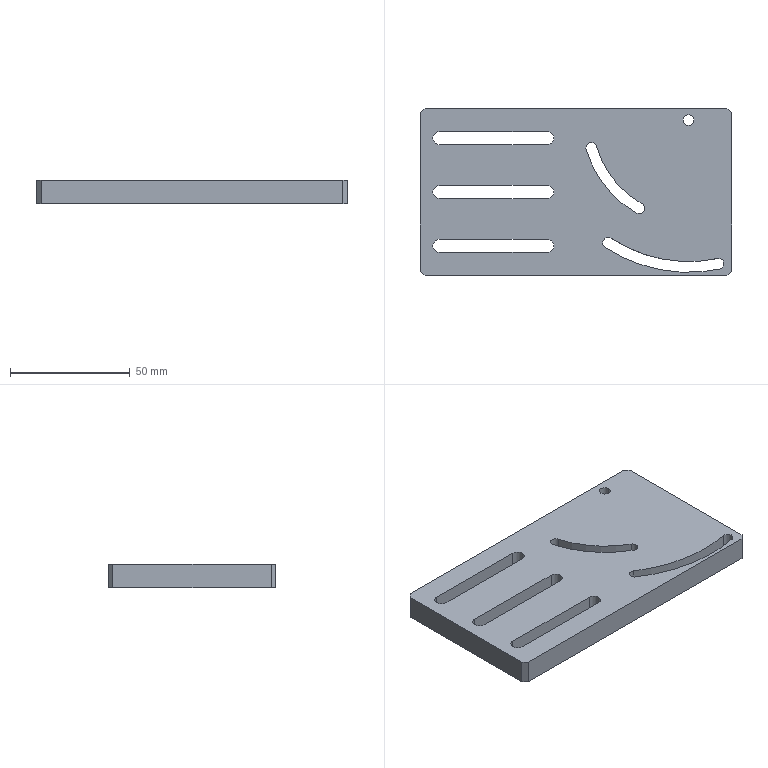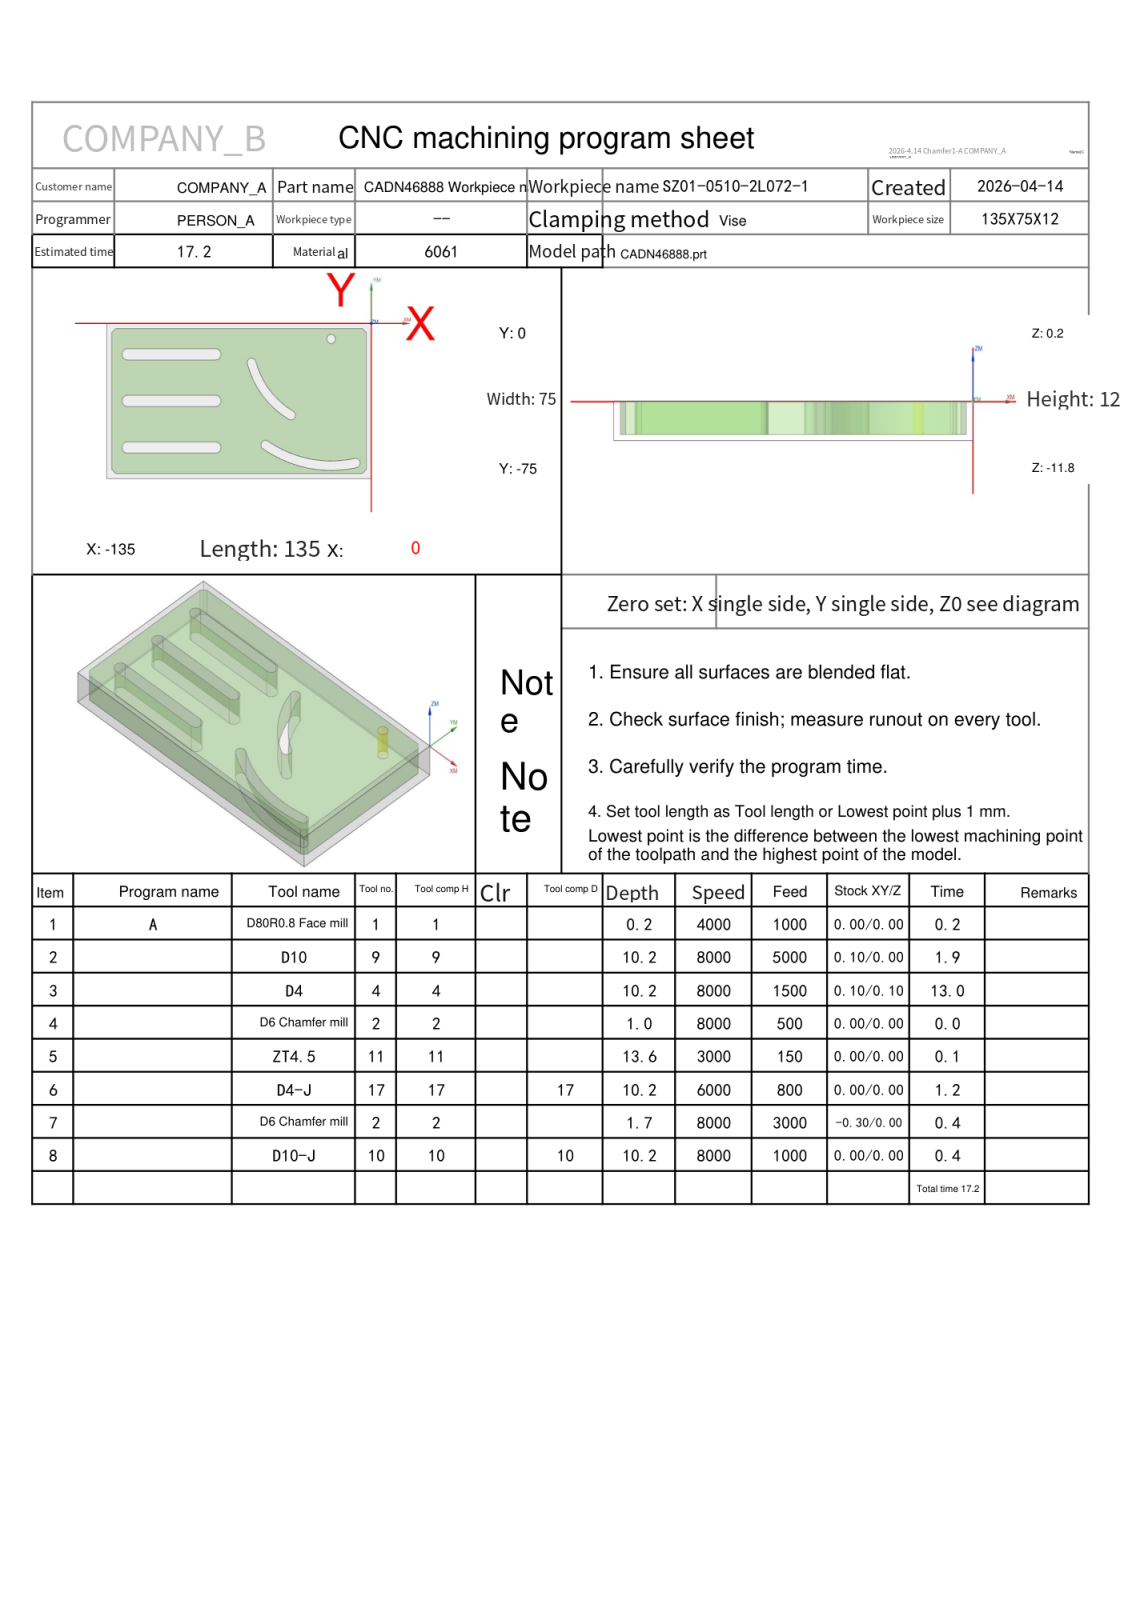NC program | NX | posted by the shop | part box 130 x 70 x 10 mm
Lines 1 to 447 of 2533:
%
O0001
(Machine time: 14.74 MIN)
(===Total Tool:7===)
(T1=D80R0.8 Face mill D=80.  R=0.8  D-  H01 Z=0.    )
(T9=D10     D=10.  R=0.   D-  H09 Z=-10.  )
(T2=D6 Chamfer mill   D=6.   R=0.   D-  H02 Z=-1.5  )
(T11=ZT4.5  D=4.5  DR_a=118 D-  H11 Z=-13.35)
(T4=D4      D=4.   R=0.   D-  H04 Z=-10.  )
(T17=D4-J   D=4.   R=0.   D17 H17 Z=-10.  )
(T10=D10-J  D=10.  R=0.   D10 H10 Z=-10.  )
G80 G90 G17 G49 G40
G91 G28 Z0
M01
N1 T01 M06
(D80R0.8 Face mill  D=80. R=0.8 H=01 ce=0.00 di=0.00)
G00 G90 G54 X-177.5 Y-37.5 M03 S4000
G43 H01 Z20.
M08
Z2.
G01 Z0.0 F1000.
X-172.5
X37.5
X42.5
Z2.
G00 Z20.
G91 G28 Z0.0
M05
M09
G91 G28 Z0.0
M01
N2 T09 M06
(D10  D=10. R=0. H=09 ce=0.10 di=0.00)
G00 G90 G54 X-67.5 Y2.6 M03 S8000
G43 H09 Z20.
M08
Z.5
G01 X-4.5 Z.426 F5000.
G02 X-.894 Y1.106 Z.422 I0.0 J-5.1
G01 X1.106 Y-.894 Z.418
G02 X2.6 Y-4.5 Z.414 I-3.606 J-3.606
G01 Y-70.5 Z.336
G02 X1.106 Y-74.106 Z.332 I-5.1 J0.0
G01 X-.894 Y-76.106 Z.328
G02 X-4.5 Y-77.6 Z.324 I-3.606 J3.606
G01 X-130.5 Z.176
G02 X-134.106 Y-76.106 Z.172 I0.0 J5.1
G01 X-136.106 Y-74.106 Z.168
G02 X-137.6 Y-70.5 Z.164 I3.606 J3.606
G01 Y-4.5 Z.086
G02 X-136.106 Y-.894 Z.082 I5.1 J0.0
G01 X-134.106 Y1.106 Z.078
G02 X-130.5 Y2.6 Z.074 I3.606 J-3.606
G01 X-4.5 Z-.074
G02 X-.894 Y1.106 Z-.078 I0.0 J-5.1
G01 X1.106 Y-.894 Z-.082
G02 X2.6 Y-4.5 Z-.086 I-3.606 J-3.606
G01 Y-70.5 Z-.164
G02 X1.106 Y-74.106 Z-.168 I-5.1 J0.0
G01 X-.894 Y-76.106 Z-.172
G02 X-4.5 Y-77.6 Z-.176 I-3.606 J3.606
G01 X-130.5 Z-.324
G02 X-134.106 Y-76.106 Z-.328 I0.0 J5.1
G01 X-136.106 Y-74.106 Z-.332
G02 X-137.6 Y-70.5 Z-.336 I3.606 J3.606
G01 Y-4.5 Z-.414
G02 X-136.106 Y-.894 Z-.418 I5.1 J0.0
G01 X-134.106 Y1.106 Z-.422
G02 X-130.5 Y2.6 Z-.426 I3.606 J-3.606
G01 X-4.5 Z-.574
G02 X-.894 Y1.106 Z-.578 I0.0 J-5.1
G01 X1.106 Y-.894 Z-.582
G02 X2.6 Y-4.5 Z-.586 I-3.606 J-3.606
G01 Y-70.5 Z-.664
G02 X1.106 Y-74.106 Z-.668 I-5.1 J0.0
G01 X-.894 Y-76.106 Z-.672
G02 X-4.5 Y-77.6 Z-.676 I-3.606 J3.606
G01 X-130.5 Z-.824
G02 X-134.106 Y-76.106 Z-.828 I0.0 J5.1
G01 X-136.106 Y-74.106 Z-.832
G02 X-137.6 Y-70.5 Z-.836 I3.606 J3.606
G01 Y-4.5 Z-.914
G02 X-136.106 Y-.894 Z-.918 I5.1 J0.0
G01 X-134.106 Y1.106 Z-.922
G02 X-130.5 Y2.6 Z-.926 I3.606 J-3.606
G01 X-4.5 Z-1.074
G02 X-.894 Y1.106 Z-1.078 I0.0 J-5.1
G01 X1.106 Y-.894 Z-1.082
G02 X2.6 Y-4.5 Z-1.086 I-3.606 J-3.606
G01 Y-70.5 Z-1.164
G02 X1.106 Y-74.106 Z-1.168 I-5.1 J0.0
G01 X-.894 Y-76.106 Z-1.172
G02 X-4.5 Y-77.6 Z-1.176 I-3.606 J3.606
G01 X-130.5 Z-1.324
G02 X-134.106 Y-76.106 Z-1.328 I0.0 J5.1
G01 X-136.106 Y-74.106 Z-1.332
G02 X-137.6 Y-70.5 Z-1.336 I3.606 J3.606
G01 Y-4.5 Z-1.414
G02 X-136.106 Y-.894 Z-1.418 I5.1 J0.0
G01 X-134.106 Y1.106 Z-1.422
G02 X-130.5 Y2.6 Z-1.426 I3.606 J-3.606
G01 X-4.5 Z-1.574
G02 X-.894 Y1.106 Z-1.578 I0.0 J-5.1
G01 X1.106 Y-.894 Z-1.582
G02 X2.6 Y-4.5 Z-1.586 I-3.606 J-3.606
G01 Y-70.5 Z-1.664
G02 X1.106 Y-74.106 Z-1.668 I-5.1 J0.0
G01 X-.894 Y-76.106 Z-1.672
G02 X-4.5 Y-77.6 Z-1.676 I-3.606 J3.606
G01 X-130.5 Z-1.824
G02 X-134.106 Y-76.106 Z-1.828 I0.0 J5.1
G01 X-136.106 Y-74.106 Z-1.832
G02 X-137.6 Y-70.5 Z-1.836 I3.606 J3.606
G01 Y-4.5 Z-1.914
G02 X-136.106 Y-.894 Z-1.918 I5.1 J0.0
G01 X-134.106 Y1.106 Z-1.922
G02 X-130.5 Y2.6 Z-1.926 I3.606 J-3.606
G01 X-4.5 Z-2.074
G02 X-.894 Y1.106 Z-2.078 I0.0 J-5.1
G01 X1.106 Y-.894 Z-2.082
G02 X2.6 Y-4.5 Z-2.086 I-3.606 J-3.606
G01 Y-70.5 Z-2.164
G02 X1.106 Y-74.106 Z-2.168 I-5.1 J0.0
G01 X-.894 Y-76.106 Z-2.172
G02 X-4.5 Y-77.6 Z-2.176 I-3.606 J3.606
G01 X-130.5 Z-2.324
G02 X-134.106 Y-76.106 Z-2.328 I0.0 J5.1
G01 X-136.106 Y-74.106 Z-2.332
G02 X-137.6 Y-70.5 Z-2.336 I3.606 J3.606
G01 Y-4.5 Z-2.414
G02 X-136.106 Y-.894 Z-2.418 I5.1 J0.0
G01 X-134.106 Y1.106 Z-2.422
G02 X-130.5 Y2.6 Z-2.426 I3.606 J-3.606
G01 X-4.5 Z-2.574
G02 X-.894 Y1.106 Z-2.578 I0.0 J-5.1
G01 X1.106 Y-.894 Z-2.582
G02 X2.6 Y-4.5 Z-2.586 I-3.606 J-3.606
G01 Y-70.5 Z-2.664
G02 X1.106 Y-74.106 Z-2.668 I-5.1 J0.0
G01 X-.894 Y-76.106 Z-2.672
G02 X-4.5 Y-77.6 Z-2.676 I-3.606 J3.606
G01 X-130.5 Z-2.824
G02 X-134.106 Y-76.106 Z-2.828 I0.0 J5.1
G01 X-136.106 Y-74.106 Z-2.832
G02 X-137.6 Y-70.5 Z-2.836 I3.606 J3.606
G01 Y-4.5 Z-2.914
G02 X-136.106 Y-.894 Z-2.918 I5.1 J0.0
G01 X-134.106 Y1.106 Z-2.922
G02 X-130.5 Y2.6 Z-2.926 I3.606 J-3.606
G01 X-4.5 Z-3.074
G02 X-.894 Y1.106 Z-3.078 I0.0 J-5.1
G01 X1.106 Y-.894 Z-3.082
G02 X2.6 Y-4.5 Z-3.086 I-3.606 J-3.606
G01 Y-70.5 Z-3.164
G02 X1.106 Y-74.106 Z-3.168 I-5.1 J0.0
G01 X-.894 Y-76.106 Z-3.172
G02 X-4.5 Y-77.6 Z-3.176 I-3.606 J3.606
G01 X-130.5 Z-3.324
G02 X-134.106 Y-76.106 Z-3.328 I0.0 J5.1
G01 X-136.106 Y-74.106 Z-3.332
G02 X-137.6 Y-70.5 Z-3.336 I3.606 J3.606
G01 Y-4.5 Z-3.414
G02 X-136.106 Y-.894 Z-3.418 I5.1 J0.0
G01 X-134.106 Y1.106 Z-3.422
G02 X-130.5 Y2.6 Z-3.426 I3.606 J-3.606
G01 X-4.5 Z-3.574
G02 X-.894 Y1.106 Z-3.578 I0.0 J-5.1
G01 X1.106 Y-.894 Z-3.582
G02 X2.6 Y-4.5 Z-3.586 I-3.606 J-3.606
G01 Y-70.5 Z-3.664
G02 X1.106 Y-74.106 Z-3.668 I-5.1 J0.0
G01 X-.894 Y-76.106 Z-3.672
G02 X-4.5 Y-77.6 Z-3.676 I-3.606 J3.606
G01 X-130.5 Z-3.824
G02 X-134.106 Y-76.106 Z-3.828 I0.0 J5.1
G01 X-136.106 Y-74.106 Z-3.832
G02 X-137.6 Y-70.5 Z-3.836 I3.606 J3.606
G01 Y-4.5 Z-3.914
G02 X-136.106 Y-.894 Z-3.918 I5.1 J0.0
G01 X-134.106 Y1.106 Z-3.922
G02 X-130.5 Y2.6 Z-3.926 I3.606 J-3.606
G01 X-4.5 Z-4.074
G02 X-.894 Y1.106 Z-4.078 I0.0 J-5.1
G01 X1.106 Y-.894 Z-4.082
G02 X2.6 Y-4.5 Z-4.086 I-3.606 J-3.606
G01 Y-70.5 Z-4.164
G02 X1.106 Y-74.106 Z-4.168 I-5.1 J0.0
G01 X-.894 Y-76.106 Z-4.172
G02 X-4.5 Y-77.6 Z-4.176 I-3.606 J3.606
G01 X-130.5 Z-4.324
G02 X-134.106 Y-76.106 Z-4.328 I0.0 J5.1
G01 X-136.106 Y-74.106 Z-4.332
G02 X-137.6 Y-70.5 Z-4.336 I3.606 J3.606
G01 Y-4.5 Z-4.414
G02 X-136.106 Y-.894 Z-4.418 I5.1 J0.0
G01 X-134.106 Y1.106 Z-4.422
G02 X-130.5 Y2.6 Z-4.426 I3.606 J-3.606
G01 X-4.5 Z-4.574
G02 X-.894 Y1.106 Z-4.578 I0.0 J-5.1
G01 X1.106 Y-.894 Z-4.582
G02 X2.6 Y-4.5 Z-4.586 I-3.606 J-3.606
G01 Y-70.5 Z-4.664
G02 X1.106 Y-74.106 Z-4.668 I-5.1 J0.0
G01 X-.894 Y-76.106 Z-4.672
G02 X-4.5 Y-77.6 Z-4.676 I-3.606 J3.606
G01 X-130.5 Z-4.824
G02 X-134.106 Y-76.106 Z-4.828 I0.0 J5.1
G01 X-136.106 Y-74.106 Z-4.832
G02 X-137.6 Y-70.5 Z-4.836 I3.606 J3.606
G01 Y-4.5 Z-4.914
G02 X-136.106 Y-.894 Z-4.918 I5.1 J0.0
G01 X-134.106 Y1.106 Z-4.922
G02 X-130.5 Y2.6 Z-4.926 I3.606 J-3.606
G01 X-4.5 Z-5.074
G02 X-.894 Y1.106 Z-5.078 I0.0 J-5.1
G01 X1.106 Y-.894 Z-5.082
G02 X2.6 Y-4.5 Z-5.086 I-3.606 J-3.606
G01 Y-70.5 Z-5.164
G02 X1.106 Y-74.106 Z-5.168 I-5.1 J0.0
G01 X-.894 Y-76.106 Z-5.172
G02 X-4.5 Y-77.6 Z-5.176 I-3.606 J3.606
G01 X-130.5 Z-5.324
G02 X-134.106 Y-76.106 Z-5.328 I0.0 J5.1
G01 X-136.106 Y-74.106 Z-5.332
G02 X-137.6 Y-70.5 Z-5.336 I3.606 J3.606
G01 Y-4.5 Z-5.414
G02 X-136.106 Y-.894 Z-5.418 I5.1 J0.0
G01 X-134.106 Y1.106 Z-5.422
G02 X-130.5 Y2.6 Z-5.426 I3.606 J-3.606
G01 X-4.5 Z-5.574
G02 X-.894 Y1.106 Z-5.578 I0.0 J-5.1
G01 X1.106 Y-.894 Z-5.582
G02 X2.6 Y-4.5 Z-5.586 I-3.606 J-3.606
G01 Y-70.5 Z-5.664
G02 X1.106 Y-74.106 Z-5.668 I-5.1 J0.0
G01 X-.894 Y-76.106 Z-5.672
G02 X-4.5 Y-77.6 Z-5.676 I-3.606 J3.606
G01 X-130.5 Z-5.824
G02 X-134.106 Y-76.106 Z-5.828 I0.0 J5.1
G01 X-136.106 Y-74.106 Z-5.832
G02 X-137.6 Y-70.5 Z-5.836 I3.606 J3.606
G01 Y-4.5 Z-5.914
G02 X-136.106 Y-.894 Z-5.918 I5.1 J0.0
G01 X-134.106 Y1.106 Z-5.922
G02 X-130.5 Y2.6 Z-5.926 I3.606 J-3.606
G01 X-4.5 Z-6.074
G02 X-.894 Y1.106 Z-6.078 I0.0 J-5.1
G01 X1.106 Y-.894 Z-6.082
G02 X2.6 Y-4.5 Z-6.086 I-3.606 J-3.606
G01 Y-70.5 Z-6.164
G02 X1.106 Y-74.106 Z-6.168 I-5.1 J0.0
G01 X-.894 Y-76.106 Z-6.172
G02 X-4.5 Y-77.6 Z-6.176 I-3.606 J3.606
G01 X-130.5 Z-6.324
G02 X-134.106 Y-76.106 Z-6.328 I0.0 J5.1
G01 X-136.106 Y-74.106 Z-6.332
G02 X-137.6 Y-70.5 Z-6.336 I3.606 J3.606
G01 Y-4.5 Z-6.414
G02 X-136.106 Y-.894 Z-6.418 I5.1 J0.0
G01 X-134.106 Y1.106 Z-6.422
G02 X-130.5 Y2.6 Z-6.426 I3.606 J-3.606
G01 X-4.5 Z-6.574
G02 X-.894 Y1.106 Z-6.578 I0.0 J-5.1
G01 X1.106 Y-.894 Z-6.582
G02 X2.6 Y-4.5 Z-6.586 I-3.606 J-3.606
G01 Y-70.5 Z-6.664
G02 X1.106 Y-74.106 Z-6.668 I-5.1 J0.0
G01 X-.894 Y-76.106 Z-6.672
G02 X-4.5 Y-77.6 Z-6.676 I-3.606 J3.606
G01 X-130.5 Z-6.824
G02 X-134.106 Y-76.106 Z-6.828 I0.0 J5.1
G01 X-136.106 Y-74.106 Z-6.832
G02 X-137.6 Y-70.5 Z-6.836 I3.606 J3.606
G01 Y-4.5 Z-6.914
G02 X-136.106 Y-.894 Z-6.918 I5.1 J0.0
G01 X-134.106 Y1.106 Z-6.922
G02 X-130.5 Y2.6 Z-6.926 I3.606 J-3.606
G01 X-4.5 Z-7.074
G02 X-.894 Y1.106 Z-7.078 I0.0 J-5.1
G01 X1.106 Y-.894 Z-7.082
G02 X2.6 Y-4.5 Z-7.086 I-3.606 J-3.606
G01 Y-70.5 Z-7.164
G02 X1.106 Y-74.106 Z-7.168 I-5.1 J0.0
G01 X-.894 Y-76.106 Z-7.172
G02 X-4.5 Y-77.6 Z-7.176 I-3.606 J3.606
G01 X-130.5 Z-7.324
G02 X-134.106 Y-76.106 Z-7.328 I0.0 J5.1
G01 X-136.106 Y-74.106 Z-7.332
G02 X-137.6 Y-70.5 Z-7.336 I3.606 J3.606
G01 Y-4.5 Z-7.414
G02 X-136.106 Y-.894 Z-7.418 I5.1 J0.0
G01 X-134.106 Y1.106 Z-7.422
G02 X-130.5 Y2.6 Z-7.426 I3.606 J-3.606
G01 X-4.5 Z-7.574
G02 X-.894 Y1.106 Z-7.578 I0.0 J-5.1
G01 X1.106 Y-.894 Z-7.582
G02 X2.6 Y-4.5 Z-7.586 I-3.606 J-3.606
G01 Y-70.5 Z-7.664
G02 X1.106 Y-74.106 Z-7.668 I-5.1 J0.0
G01 X-.894 Y-76.106 Z-7.672
G02 X-4.5 Y-77.6 Z-7.676 I-3.606 J3.606
G01 X-130.5 Z-7.824
G02 X-134.106 Y-76.106 Z-7.828 I0.0 J5.1
G01 X-136.106 Y-74.106 Z-7.832
G02 X-137.6 Y-70.5 Z-7.836 I3.606 J3.606
G01 Y-4.5 Z-7.914
G02 X-136.106 Y-.894 Z-7.918 I5.1 J0.0
G01 X-134.106 Y1.106 Z-7.922
G02 X-130.5 Y2.6 Z-7.926 I3.606 J-3.606
G01 X-4.5 Z-8.074
G02 X-.894 Y1.106 Z-8.078 I0.0 J-5.1
G01 X1.106 Y-.894 Z-8.082
G02 X2.6 Y-4.5 Z-8.086 I-3.606 J-3.606
G01 Y-70.5 Z-8.164
G02 X1.106 Y-74.106 Z-8.168 I-5.1 J0.0
G01 X-.894 Y-76.106 Z-8.172
G02 X-4.5 Y-77.6 Z-8.176 I-3.606 J3.606
G01 X-130.5 Z-8.324
G02 X-134.106 Y-76.106 Z-8.328 I0.0 J5.1
G01 X-136.106 Y-74.106 Z-8.332
G02 X-137.6 Y-70.5 Z-8.336 I3.606 J3.606
G01 Y-4.5 Z-8.414
G02 X-136.106 Y-.894 Z-8.418 I5.1 J0.0
G01 X-134.106 Y1.106 Z-8.422
G02 X-130.5 Y2.6 Z-8.426 I3.606 J-3.606
G01 X-4.5 Z-8.574
G02 X-.894 Y1.106 Z-8.578 I0.0 J-5.1
G01 X1.106 Y-.894 Z-8.582
G02 X2.6 Y-4.5 Z-8.586 I-3.606 J-3.606
G01 Y-70.5 Z-8.664
G02 X1.106 Y-74.106 Z-8.668 I-5.1 J0.0
G01 X-.894 Y-76.106 Z-8.672
G02 X-4.5 Y-77.6 Z-8.676 I-3.606 J3.606
G01 X-130.5 Z-8.824
G02 X-134.106 Y-76.106 Z-8.828 I0.0 J5.1
G01 X-136.106 Y-74.106 Z-8.832
G02 X-137.6 Y-70.5 Z-8.836 I3.606 J3.606
G01 Y-4.5 Z-8.914
G02 X-136.106 Y-.894 Z-8.918 I5.1 J0.0
G01 X-134.106 Y1.106 Z-8.922
G02 X-130.5 Y2.6 Z-8.926 I3.606 J-3.606
G01 X-4.5 Z-9.074
G02 X-.894 Y1.106 Z-9.078 I0.0 J-5.1
G01 X1.106 Y-.894 Z-9.082
G02 X2.6 Y-4.5 Z-9.086 I-3.606 J-3.606
G01 Y-70.5 Z-9.164
G02 X1.106 Y-74.106 Z-9.168 I-5.1 J0.0
G01 X-.894 Y-76.106 Z-9.172
G02 X-4.5 Y-77.6 Z-9.176 I-3.606 J3.606
G01 X-130.5 Z-9.324
G02 X-134.106 Y-76.106 Z-9.328 I0.0 J5.1
G01 X-136.106 Y-74.106 Z-9.332
G02 X-137.6 Y-70.5 Z-9.336 I3.606 J3.606
G01 Y-4.5 Z-9.414
G02 X-136.106 Y-.894 Z-9.418 I5.1 J0.0
G01 X-134.106 Y1.106 Z-9.422
G02 X-130.5 Y2.6 Z-9.426 I3.606 J-3.606
G01 X-4.5 Z-9.574
G02 X-.894 Y1.106 Z-9.578 I0.0 J-5.1
G01 X1.106 Y-.894 Z-9.582
G02 X2.6 Y-4.5 Z-9.586 I-3.606 J-3.606
G01 Y-70.5 Z-9.664
G02 X1.106 Y-74.106 Z-9.668 I-5.1 J0.0
G01 X-.894 Y-76.106 Z-9.672
G02 X-4.5 Y-77.6 Z-9.676 I-3.606 J3.606
G01 X-130.5 Z-9.824
G02 X-134.106 Y-76.106 Z-9.828 I0.0 J5.1
G01 X-136.106 Y-74.106 Z-9.832
G02 X-137.6 Y-70.5 Z-9.836 I3.606 J3.606
G01 Y-4.5 Z-9.914
G02 X-136.106 Y-.894 Z-9.918 I5.1 J0.0
G01 X-134.106 Y1.106 Z-9.922
G02 X-130.5 Y2.6 Z-9.926 I3.606 J-3.606
G01 X-67.5 Z-10.
X-4.5
G02 X-.894 Y1.106 I0.0 J-5.1
G01 X1.106 Y-.894
G02 X2.6 Y-4.5 I-3.606 J-3.606
G01 Y-70.5
G02 X1.106 Y-74.106 I-5.1 J0.0
G01 X-.894 Y-76.106
G02 X-4.5 Y-77.6 I-3.606 J3.606
G01 X-130.5
G02 X-134.106 Y-76.106 I0.0 J5.1
G01 X-136.106 Y-74.106
G02 X-137.6 Y-70.5 I3.606 J3.606
G01 Y-4.5
G02 X-136.106 Y-.894 I5.1 J0.0
G01 X-134.106 Y1.106
G02 X-130.5 Y2.6 I3.606 J-3.606
G01 X-67.5
X-67.
Z-9.
G00 Z20.
G91 G28 Z0.0
M05
M09
G91 G28 Z0.0
M01
N3 T02 M06
(D6 Chamfer mill  D=6. R=0. H=02 ce=0.00 di=0.00)
G00 G90 G54 X-20.5 Y-7.5 M03 S8000
G43 H02 Z20.
M08
G98 G81 X-20.5 Y-7.5 Z-.8 R1. F500.
X-124.5 Y-15.
X-79.5
X-61.088 Y-19.097
X-41. Y-44.4
X-54.088 Y-58.765
X-8. Y-67.5
X-79.5 Y-37.5
X-124.5
Y-60.
X-79.5
G80
G00 Z20.
G91 G28 Z0.0
M05
M09
G91 G28 Z0.0
M01
N4 T11 M06
(ZT4.5 D=4.5 DR_a=118 H=11)
G00 G90 G54 X-20.5 Y-7.5 M03 S3000
G43 H11 Z20.
M08
G98 G83 X-20.5 Y-7.5 Z-13.352 R1. F150. Q3.
X-61.088 Y-19.097
X-41. Y-44.4
X-8. Y-67.5
X-54.088 Y-58.765
X-124.5 Y-60.
X-79.5
Y-37.5
X-124.5
Y-15.
X-79.5
G80
G00 Z20.
G91 G28 Z0.0
M05
M09
G91 G28 Z0.0
M01